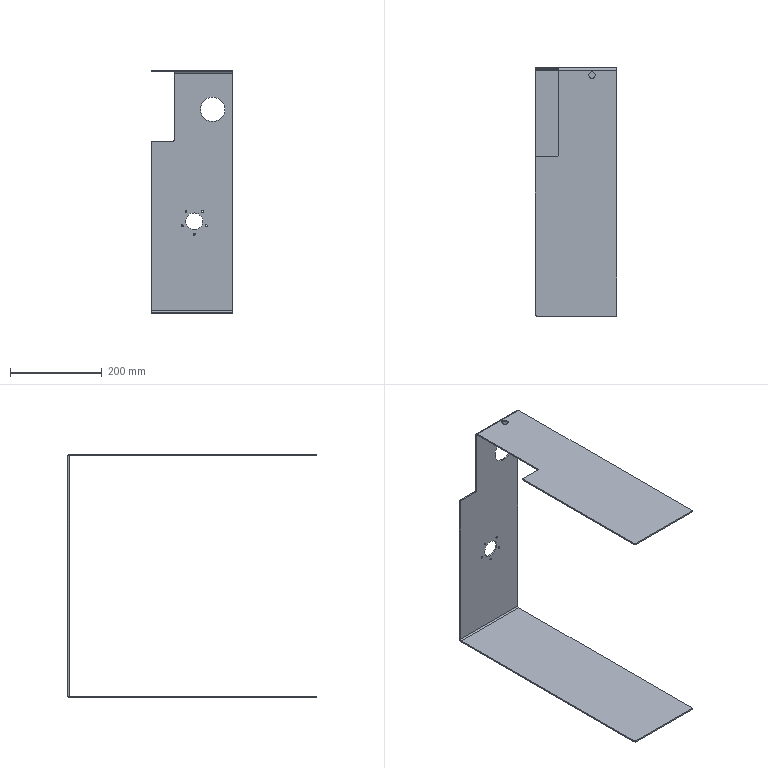Part | SolidWorks | features ICE 3, Fillet 2, FlatPattern 1, HoleWzd 1, SMBaseFlange 1, SheetMetal 1 | 1 solid | 46 faces | box 177 x 542 x 530 mm | volume 789505 mm3 | cylinder 24 | plane 22 | commonest cylinder face diameters 4.2 x10 6 x2 7 x2 8 x2 12 x2 14.2 x2
STEP:
#1=CARTESIAN_POINT('',(93.5,539.,-359.1));
#2=VERTEX_POINT('',#1);
#3=CARTESIAN_POINT('',(93.5,539.,-354.9));
#4=VERTEX_POINT('',#3);
#5=CARTESIAN_POINT('',(93.5,539.,-357.));
#6=DIRECTION('',(0.,1.,0.));
#7=DIRECTION('',(0.,0.,1.));
#8=AXIS2_PLACEMENT_3D('',#5,#6,#7);
#9=CIRCLE('',#8,2.1);
#10=EDGE_CURVE('',#2,#4,#9,.T.);
#11=ORIENTED_EDGE('',*,*,#10,.F.);
#12=CARTESIAN_POINT('',(93.5,542.,-359.1));
#13=VERTEX_POINT('',#12);
#14=CARTESIAN_POINT('',(93.5,542.,-359.1));
#15=DIRECTION('',(0.,1.,0.));
#16=VECTOR('',#15,1000.);
#17=LINE('',#14,#16);
#18=EDGE_CURVE('',#2,#13,#17,.T.);
#19=ORIENTED_EDGE('',*,*,#18,.T.);
#20=CARTESIAN_POINT('',(93.5,542.,-354.9));
#21=VERTEX_POINT('',#20);
#22=CARTESIAN_POINT('',(93.5,542.,-357.));
#23=DIRECTION('',(0.,1.,0.));
#24=DIRECTION('',(0.,0.,1.));
#25=AXIS2_PLACEMENT_3D('',#22,#23,#24);
#26=CIRCLE('',#25,2.1);
#27=EDGE_CURVE('',#13,#21,#26,.T.);
#28=ORIENTED_EDGE('',*,*,#27,.T.);
#29=CARTESIAN_POINT('',(93.5,542.,-354.9));
#30=DIRECTION('',(0.,1.,0.));
#31=VECTOR('',#30,1000.);
#32=LINE('',#29,#31);
#33=EDGE_CURVE('',#4,#21,#32,.T.);
#34=ORIENTED_EDGE('',*,*,#33,.F.);
#35=EDGE_LOOP('',(#11,#19,#28,#34));
#36=FACE_OUTER_BOUND('',#35,.T.);
#37=CARTESIAN_POINT('',(93.5,542.,-357.));
#38=DIRECTION('',(0.,1.,0.));
#39=DIRECTION('',(0.,0.,1.));
#40=AXIS2_PLACEMENT_3D('',#37,#38,#39);
#41=CYLINDRICAL_SURFACE('',#40,2.1);
#42=ADVANCED_FACE('',(#36),#41,.F.);
#43=CARTESIAN_POINT('',(119.811,539.,-340.677));
#44=VERTEX_POINT('',#43);
#45=CARTESIAN_POINT('',(119.811,539.,-336.477));
#46=VERTEX_POINT('',#45);
#47=CARTESIAN_POINT('',(119.811,539.,-338.577));
#48=DIRECTION('',(0.,1.,0.));
#49=DIRECTION('',(0.,0.,1.));
#50=AXIS2_PLACEMENT_3D('',#47,#48,#49);
#51=CIRCLE('',#50,2.1);
#52=EDGE_CURVE('',#44,#46,#51,.T.);
#53=ORIENTED_EDGE('',*,*,#52,.F.);
#54=CARTESIAN_POINT('',(119.811,542.,-340.677));
#55=VERTEX_POINT('',#54);
#56=CARTESIAN_POINT('',(119.811,542.,-340.677));
#57=DIRECTION('',(0.,1.,0.));
#58=VECTOR('',#57,1000.);
#59=LINE('',#56,#58);
#60=EDGE_CURVE('',#44,#55,#59,.T.);
#61=ORIENTED_EDGE('',*,*,#60,.T.);
#62=CARTESIAN_POINT('',(119.811,542.,-336.477));
#63=VERTEX_POINT('',#62);
#64=CARTESIAN_POINT('',(119.811,542.,-338.577));
#65=DIRECTION('',(0.,1.,0.));
#66=DIRECTION('',(0.,0.,1.));
#67=AXIS2_PLACEMENT_3D('',#64,#65,#66);
#68=CIRCLE('',#67,2.1);
#69=EDGE_CURVE('',#55,#63,#68,.T.);
#70=ORIENTED_EDGE('',*,*,#69,.T.);
#71=CARTESIAN_POINT('',(119.811,542.,-336.477));
#72=DIRECTION('',(0.,1.,0.));
#73=VECTOR('',#72,1000.);
#74=LINE('',#71,#73);
#75=EDGE_CURVE('',#46,#63,#74,.T.);
#76=ORIENTED_EDGE('',*,*,#75,.F.);
#77=EDGE_LOOP('',(#53,#61,#70,#76));
#78=FACE_OUTER_BOUND('',#77,.T.);
#79=CARTESIAN_POINT('',(119.811,542.,-338.577));
#80=DIRECTION('',(0.,1.,0.));
#81=DIRECTION('',(0.,0.,1.));
#82=AXIS2_PLACEMENT_3D('',#79,#80,#81);
#83=CYLINDRICAL_SURFACE('',#82,2.1);
#84=ADVANCED_FACE('',(#78),#83,.F.);
#85=CARTESIAN_POINT('',(111.498,539.,-309.651));
#86=VERTEX_POINT('',#85);
#87=CARTESIAN_POINT('',(111.498,539.,-305.451));
#88=VERTEX_POINT('',#87);
#89=CARTESIAN_POINT('',(111.498,539.,-307.551));
#90=DIRECTION('',(0.,1.,0.));
#91=DIRECTION('',(0.,0.,1.));
#92=AXIS2_PLACEMENT_3D('',#89,#90,#91);
#93=CIRCLE('',#92,2.1);
#94=EDGE_CURVE('',#86,#88,#93,.T.);
#95=ORIENTED_EDGE('',*,*,#94,.F.);
#96=CARTESIAN_POINT('',(111.498,542.,-309.651));
#97=VERTEX_POINT('',#96);
#98=CARTESIAN_POINT('',(111.498,542.,-309.651));
#99=DIRECTION('',(0.,1.,0.));
#100=VECTOR('',#99,1000.);
#101=LINE('',#98,#100);
#102=EDGE_CURVE('',#86,#97,#101,.T.);
#103=ORIENTED_EDGE('',*,*,#102,.T.);
#104=CARTESIAN_POINT('',(111.498,542.,-305.451));
#105=VERTEX_POINT('',#104);
#106=CARTESIAN_POINT('',(111.498,542.,-307.551));
#107=DIRECTION('',(0.,1.,0.));
#108=DIRECTION('',(0.,0.,1.));
#109=AXIS2_PLACEMENT_3D('',#106,#107,#108);
#110=CIRCLE('',#109,2.1);
#111=EDGE_CURVE('',#97,#105,#110,.T.);
#112=ORIENTED_EDGE('',*,*,#111,.T.);
#113=CARTESIAN_POINT('',(111.498,542.,-305.451));
#114=DIRECTION('',(0.,1.,0.));
#115=VECTOR('',#114,1000.);
#116=LINE('',#113,#115);
#117=EDGE_CURVE('',#88,#105,#116,.T.);
#118=ORIENTED_EDGE('',*,*,#117,.F.);
#119=EDGE_LOOP('',(#95,#103,#112,#118));
#120=FACE_OUTER_BOUND('',#119,.T.);
#121=CARTESIAN_POINT('',(111.498,542.,-307.551));
#122=DIRECTION('',(0.,1.,0.));
#123=DIRECTION('',(0.,0.,1.));
#124=AXIS2_PLACEMENT_3D('',#121,#122,#123);
#125=CYLINDRICAL_SURFACE('',#124,2.1);
#126=ADVANCED_FACE('',(#120),#125,.F.);
#127=CARTESIAN_POINT('',(75.502,539.,-309.651));
#128=VERTEX_POINT('',#127);
#129=CARTESIAN_POINT('',(75.502,539.,-305.451));
#130=VERTEX_POINT('',#129);
#131=CARTESIAN_POINT('',(75.502,539.,-307.551));
#132=DIRECTION('',(0.,1.,0.));
#133=DIRECTION('',(0.,0.,1.));
#134=AXIS2_PLACEMENT_3D('',#131,#132,#133);
#135=CIRCLE('',#134,2.1);
#136=EDGE_CURVE('',#128,#130,#135,.T.);
#137=ORIENTED_EDGE('',*,*,#136,.F.);
#138=CARTESIAN_POINT('',(75.502,542.,-309.651));
#139=VERTEX_POINT('',#138);
#140=CARTESIAN_POINT('',(75.502,542.,-309.651));
#141=DIRECTION('',(0.,1.,0.));
#142=VECTOR('',#141,1000.);
#143=LINE('',#140,#142);
#144=EDGE_CURVE('',#128,#139,#143,.T.);
#145=ORIENTED_EDGE('',*,*,#144,.T.);
#146=CARTESIAN_POINT('',(75.502,542.,-305.451));
#147=VERTEX_POINT('',#146);
#148=CARTESIAN_POINT('',(75.502,542.,-307.551));
#149=DIRECTION('',(0.,1.,0.));
#150=DIRECTION('',(0.,0.,1.));
#151=AXIS2_PLACEMENT_3D('',#148,#149,#150);
#152=CIRCLE('',#151,2.1);
#153=EDGE_CURVE('',#139,#147,#152,.T.);
#154=ORIENTED_EDGE('',*,*,#153,.T.);
#155=CARTESIAN_POINT('',(75.502,542.,-305.451));
#156=DIRECTION('',(0.,1.,0.));
#157=VECTOR('',#156,1000.);
#158=LINE('',#155,#157);
#159=EDGE_CURVE('',#130,#147,#158,.T.);
#160=ORIENTED_EDGE('',*,*,#159,.F.);
#161=EDGE_LOOP('',(#137,#145,#154,#160));
#162=FACE_OUTER_BOUND('',#161,.T.);
#163=CARTESIAN_POINT('',(75.502,542.,-307.551));
#164=DIRECTION('',(0.,1.,0.));
#165=DIRECTION('',(0.,0.,1.));
#166=AXIS2_PLACEMENT_3D('',#163,#164,#165);
#167=CYLINDRICAL_SURFACE('',#166,2.1);
#168=ADVANCED_FACE('',(#162),#167,.F.);
#169=CARTESIAN_POINT('',(67.189,539.,-340.677));
#170=VERTEX_POINT('',#169);
#171=CARTESIAN_POINT('',(67.189,539.,-336.477));
#172=VERTEX_POINT('',#171);
#173=CARTESIAN_POINT('',(67.189,539.,-338.577));
#174=DIRECTION('',(0.,1.,0.));
#175=DIRECTION('',(0.,0.,1.));
#176=AXIS2_PLACEMENT_3D('',#173,#174,#175);
#177=CIRCLE('',#176,2.1);
#178=EDGE_CURVE('',#170,#172,#177,.T.);
#179=ORIENTED_EDGE('',*,*,#178,.F.);
#180=CARTESIAN_POINT('',(67.189,542.,-340.677));
#181=VERTEX_POINT('',#180);
#182=CARTESIAN_POINT('',(67.189,542.,-340.677));
#183=DIRECTION('',(0.,1.,0.));
#184=VECTOR('',#183,1000.);
#185=LINE('',#182,#184);
#186=EDGE_CURVE('',#170,#181,#185,.T.);
#187=ORIENTED_EDGE('',*,*,#186,.T.);
#188=CARTESIAN_POINT('',(67.189,542.,-336.477));
#189=VERTEX_POINT('',#188);
#190=CARTESIAN_POINT('',(67.189,542.,-338.577));
#191=DIRECTION('',(0.,1.,0.));
#192=DIRECTION('',(0.,0.,1.));
#193=AXIS2_PLACEMENT_3D('',#190,#191,#192);
#194=CIRCLE('',#193,2.1);
#195=EDGE_CURVE('',#181,#189,#194,.T.);
#196=ORIENTED_EDGE('',*,*,#195,.T.);
#197=CARTESIAN_POINT('',(67.189,542.,-336.477));
#198=DIRECTION('',(0.,1.,0.));
#199=VECTOR('',#198,1000.);
#200=LINE('',#197,#199);
#201=EDGE_CURVE('',#172,#189,#200,.T.);
#202=ORIENTED_EDGE('',*,*,#201,.F.);
#203=EDGE_LOOP('',(#179,#187,#196,#202));
#204=FACE_OUTER_BOUND('',#203,.T.);
#205=CARTESIAN_POINT('',(67.189,542.,-338.577));
#206=DIRECTION('',(0.,1.,0.));
#207=DIRECTION('',(0.,0.,1.));
#208=AXIS2_PLACEMENT_3D('',#205,#206,#207);
#209=CYLINDRICAL_SURFACE('',#208,2.1);
#210=ADVANCED_FACE('',(#204),#209,.F.);
#211=CARTESIAN_POINT('',(133.5,539.,-58.5));
#212=VERTEX_POINT('',#211);
#213=CARTESIAN_POINT('',(133.5,539.,-111.5));
#214=VERTEX_POINT('',#213);
#215=CARTESIAN_POINT('',(133.5,539.,-85.));
#216=DIRECTION('',(0.,-1.,0.));
#217=DIRECTION('',(0.,0.,1.));
#218=AXIS2_PLACEMENT_3D('',#215,#216,#217);
#219=CIRCLE('',#218,26.5);
#220=EDGE_CURVE('',#212,#214,#219,.T.);
#221=ORIENTED_EDGE('',*,*,#220,.T.);
#222=CARTESIAN_POINT('',(133.5,542.,-111.5));
#223=VERTEX_POINT('',#222);
#224=CARTESIAN_POINT('',(133.5,-0.001,-111.5));
#225=DIRECTION('',(0.,1.,0.));
#226=VECTOR('',#225,1000.);
#227=LINE('',#224,#226);
#228=EDGE_CURVE('',#214,#223,#227,.T.);
#229=ORIENTED_EDGE('',*,*,#228,.T.);
#230=CARTESIAN_POINT('',(133.5,542.,-58.5));
#231=VERTEX_POINT('',#230);
#232=CARTESIAN_POINT('',(133.5,542.,-85.));
#233=DIRECTION('',(0.,1.,0.));
#234=DIRECTION('',(0.,0.,1.));
#235=AXIS2_PLACEMENT_3D('',#232,#233,#234);
#236=CIRCLE('',#235,26.5);
#237=EDGE_CURVE('',#223,#231,#236,.T.);
#238=ORIENTED_EDGE('',*,*,#237,.T.);
#239=CARTESIAN_POINT('',(133.5,-0.001,-58.5));
#240=DIRECTION('',(0.,1.,0.));
#241=VECTOR('',#240,1000.);
#242=LINE('',#239,#241);
#243=EDGE_CURVE('',#212,#231,#242,.T.);
#244=ORIENTED_EDGE('',*,*,#243,.F.);
#245=EDGE_LOOP('',(#221,#229,#238,#244));
#246=FACE_OUTER_BOUND('',#245,.T.);
#247=CARTESIAN_POINT('',(133.5,-0.001,-85.));
#248=DIRECTION('',(0.,1.,0.));
#249=DIRECTION('',(0.,0.,1.));
#250=AXIS2_PLACEMENT_3D('',#247,#248,#249);
#251=CYLINDRICAL_SURFACE('',#250,26.5);
#252=ADVANCED_FACE('',(#246),#251,.F.);
#253=CARTESIAN_POINT('',(93.5,539.,-310.5));
#254=VERTEX_POINT('',#253);
#255=CARTESIAN_POINT('',(93.5,539.,-347.5));
#256=VERTEX_POINT('',#255);
#257=CARTESIAN_POINT('',(93.5,539.,-329.));
#258=DIRECTION('',(0.,-1.,0.));
#259=DIRECTION('',(0.,0.,1.));
#260=AXIS2_PLACEMENT_3D('',#257,#258,#259);
#261=CIRCLE('',#260,18.5);
#262=EDGE_CURVE('',#254,#256,#261,.T.);
#263=ORIENTED_EDGE('',*,*,#262,.T.);
#264=CARTESIAN_POINT('',(93.5,542.,-347.5));
#265=VERTEX_POINT('',#264);
#266=CARTESIAN_POINT('',(93.5,-0.001,-347.5));
#267=DIRECTION('',(0.,1.,0.));
#268=VECTOR('',#267,1000.);
#269=LINE('',#266,#268);
#270=EDGE_CURVE('',#256,#265,#269,.T.);
#271=ORIENTED_EDGE('',*,*,#270,.T.);
#272=CARTESIAN_POINT('',(93.5,542.,-310.5));
#273=VERTEX_POINT('',#272);
#274=CARTESIAN_POINT('',(93.5,542.,-329.));
#275=DIRECTION('',(0.,1.,0.));
#276=DIRECTION('',(0.,0.,1.));
#277=AXIS2_PLACEMENT_3D('',#274,#275,#276);
#278=CIRCLE('',#277,18.5);
#279=EDGE_CURVE('',#265,#273,#278,.T.);
#280=ORIENTED_EDGE('',*,*,#279,.T.);
#281=CARTESIAN_POINT('',(93.5,-0.001,-310.5));
#282=DIRECTION('',(0.,1.,0.));
#283=VECTOR('',#282,1000.);
#284=LINE('',#281,#283);
#285=EDGE_CURVE('',#254,#273,#284,.T.);
#286=ORIENTED_EDGE('',*,*,#285,.F.);
#287=EDGE_LOOP('',(#263,#271,#280,#286));
#288=FACE_OUTER_BOUND('',#287,.T.);
#289=CARTESIAN_POINT('',(93.5,-0.001,-329.));
#290=DIRECTION('',(0.,1.,0.));
#291=DIRECTION('',(0.,0.,1.));
#292=AXIS2_PLACEMENT_3D('',#289,#290,#291);
#293=CYLINDRICAL_SURFACE('',#292,18.5);
#294=ADVANCED_FACE('',(#288),#293,.F.);
#295=CARTESIAN_POINT('',(130.6,525.,-3.));
#296=VERTEX_POINT('',#295);
#297=CARTESIAN_POINT('',(116.4,525.,-3.));
#298=VERTEX_POINT('',#297);
#299=CARTESIAN_POINT('',(123.5,525.,-3.));
#300=DIRECTION('',(0.,0.,-1.));
#301=DIRECTION('',(1.,0.,0.));
#302=AXIS2_PLACEMENT_3D('',#299,#300,#301);
#303=CIRCLE('',#302,7.1);
#304=EDGE_CURVE('',#296,#298,#303,.T.);
#305=ORIENTED_EDGE('',*,*,#304,.T.);
#306=CARTESIAN_POINT('',(116.4,525.,0.));
#307=VERTEX_POINT('',#306);
#308=CARTESIAN_POINT('',(116.4,525.,-530.001));
#309=DIRECTION('',(0.,0.,1.));
#310=VECTOR('',#309,1000.);
#311=LINE('',#308,#310);
#312=EDGE_CURVE('',#298,#307,#311,.T.);
#313=ORIENTED_EDGE('',*,*,#312,.T.);
#314=CARTESIAN_POINT('',(130.6,525.,0.));
#315=VERTEX_POINT('',#314);
#316=CARTESIAN_POINT('',(123.5,525.,0.));
#317=DIRECTION('',(0.,0.,1.));
#318=DIRECTION('',(1.,0.,0.));
#319=AXIS2_PLACEMENT_3D('',#316,#317,#318);
#320=CIRCLE('',#319,7.1);
#321=EDGE_CURVE('',#307,#315,#320,.T.);
#322=ORIENTED_EDGE('',*,*,#321,.T.);
#323=CARTESIAN_POINT('',(130.6,525.,-530.001));
#324=DIRECTION('',(0.,0.,1.));
#325=VECTOR('',#324,1000.);
#326=LINE('',#323,#325);
#327=EDGE_CURVE('',#296,#315,#326,.T.);
#328=ORIENTED_EDGE('',*,*,#327,.F.);
#329=EDGE_LOOP('',(#305,#313,#322,#328));
#330=FACE_OUTER_BOUND('',#329,.T.);
#331=CARTESIAN_POINT('',(123.5,525.,-530.001));
#332=DIRECTION('',(0.,0.,1.));
#333=DIRECTION('',(1.,0.,0.));
#334=AXIS2_PLACEMENT_3D('',#331,#332,#333);
#335=CYLINDRICAL_SURFACE('',#334,7.1);
#336=ADVANCED_FACE('',(#330),#335,.F.);
#337=CARTESIAN_POINT('',(50.,542.,-6.));
#338=VERTEX_POINT('',#337);
#339=CARTESIAN_POINT('',(50.,542.,-151.5));
#340=VERTEX_POINT('',#339);
#341=CARTESIAN_POINT('',(50.,542.,-155.));
#342=DIRECTION('',(0.,0.,-1.));
#343=VECTOR('',#342,1000.);
#344=LINE('',#341,#343);
#345=EDGE_CURVE('',#338,#340,#344,.T.);
#346=ORIENTED_EDGE('',*,*,#345,.T.);
#347=CARTESIAN_POINT('',(50.,539.,-151.5));
#348=VERTEX_POINT('',#347);
#349=CARTESIAN_POINT('',(50.,539.,-151.5));
#350=DIRECTION('',(0.,-1.,0.));
#351=VECTOR('',#350,1000.);
#352=LINE('',#349,#351);
#353=EDGE_CURVE('',#340,#348,#352,.T.);
#354=ORIENTED_EDGE('',*,*,#353,.T.);
#355=CARTESIAN_POINT('',(50.,539.,-6.));
#356=VERTEX_POINT('',#355);
#357=CARTESIAN_POINT('',(50.,539.,0.));
#358=DIRECTION('',(0.,0.,-1.));
#359=VECTOR('',#358,1000.);
#360=LINE('',#357,#359);
#361=EDGE_CURVE('',#356,#348,#360,.T.);
#362=ORIENTED_EDGE('',*,*,#361,.F.);
#363=CARTESIAN_POINT('',(50.,539.,-6.));
#364=DIRECTION('',(0.,1.,0.));
#365=VECTOR('',#364,1000.);
#366=LINE('',#363,#365);
#367=EDGE_CURVE('',#356,#338,#366,.T.);
#368=ORIENTED_EDGE('',*,*,#367,.T.);
#369=EDGE_LOOP('',(#346,#354,#362,#368));
#370=FACE_OUTER_BOUND('',#369,.T.);
#371=CARTESIAN_POINT('',(50.,347.,-155.));
#372=DIRECTION('',(1.,0.,0.));
#373=DIRECTION('',(0.,0.,-1.));
#374=AXIS2_PLACEMENT_3D('',#371,#372,#373);
#375=PLANE('',#374);
#376=ADVANCED_FACE('',(#370),#375,.F.);
#377=CARTESIAN_POINT('',(50.,350.5,-3.));
#378=VERTEX_POINT('',#377);
#379=CARTESIAN_POINT('',(50.,536.,-3.));
#380=VERTEX_POINT('',#379);
#381=CARTESIAN_POINT('',(50.,0.,-3.));
#382=DIRECTION('',(0.,1.,0.));
#383=VECTOR('',#382,1000.);
#384=LINE('',#381,#383);
#385=EDGE_CURVE('',#378,#380,#384,.T.);
#386=ORIENTED_EDGE('',*,*,#385,.F.);
#387=CARTESIAN_POINT('',(50.,350.5,0.));
#388=VERTEX_POINT('',#387);
#389=CARTESIAN_POINT('',(50.,350.5,0.));
#390=DIRECTION('',(0.,0.,1.));
#391=VECTOR('',#390,1000.);
#392=LINE('',#389,#391);
#393=EDGE_CURVE('',#378,#388,#392,.T.);
#394=ORIENTED_EDGE('',*,*,#393,.T.);
#395=CARTESIAN_POINT('',(50.,536.,0.));
#396=VERTEX_POINT('',#395);
#397=CARTESIAN_POINT('',(50.,347.,0.));
#398=DIRECTION('',(0.,1.,0.));
#399=VECTOR('',#398,1000.);
#400=LINE('',#397,#399);
#401=EDGE_CURVE('',#388,#396,#400,.T.);
#402=ORIENTED_EDGE('',*,*,#401,.T.);
#403=CARTESIAN_POINT('',(50.,536.,0.));
#404=DIRECTION('',(0.,0.,-1.));
#405=VECTOR('',#404,1000.);
#406=LINE('',#403,#405);
#407=EDGE_CURVE('',#396,#380,#406,.T.);
#408=ORIENTED_EDGE('',*,*,#407,.T.);
#409=EDGE_LOOP('',(#386,#394,#402,#408));
#410=FACE_OUTER_BOUND('',#409,.T.);
#411=CARTESIAN_POINT('',(50.,347.,-155.));
#412=DIRECTION('',(1.,0.,0.));
#413=DIRECTION('',(0.,0.,-1.));
#414=AXIS2_PLACEMENT_3D('',#411,#412,#413);
#415=PLANE('',#414);
#416=ADVANCED_FACE('',(#410),#415,.F.);
#417=CARTESIAN_POINT('',(177.,542.,-6.));
#418=VERTEX_POINT('',#417);
#419=CARTESIAN_POINT('',(177.,539.,-6.));
#420=VERTEX_POINT('',#419);
#421=CARTESIAN_POINT('',(177.,542.,-6.));
#422=DIRECTION('',(0.,-1.,0.));
#423=VECTOR('',#422,1000.);
#424=LINE('',#421,#423);
#425=EDGE_CURVE('',#418,#420,#424,.T.);
#426=ORIENTED_EDGE('',*,*,#425,.F.);
#427=CARTESIAN_POINT('',(177.,536.,0.));
#428=VERTEX_POINT('',#427);
#429=CARTESIAN_POINT('',(177.,536.,-6.));
#430=DIRECTION('',(-1.,0.,0.));
#431=DIRECTION('',(0.,0.,-1.));
#432=AXIS2_PLACEMENT_3D('',#429,#430,#431);
#433=CIRCLE('',#432,6.);
#434=EDGE_CURVE('',#428,#418,#433,.T.);
#435=ORIENTED_EDGE('',*,*,#434,.F.);
#436=CARTESIAN_POINT('',(177.,536.,-3.));
#437=VERTEX_POINT('',#436);
#438=CARTESIAN_POINT('',(177.,536.,-3.));
#439=DIRECTION('',(0.,0.,1.));
#440=VECTOR('',#439,1000.);
#441=LINE('',#438,#440);
#442=EDGE_CURVE('',#437,#428,#441,.T.);
#443=ORIENTED_EDGE('',*,*,#442,.F.);
#444=CARTESIAN_POINT('',(177.,536.,-6.));
#445=DIRECTION('',(-1.,0.,0.));
#446=DIRECTION('',(0.,0.,-1.));
#447=AXIS2_PLACEMENT_3D('',#444,#445,#446);
#448=CIRCLE('',#447,3.);
#449=EDGE_CURVE('',#437,#420,#448,.T.);
#450=ORIENTED_EDGE('',*,*,#449,.T.);
#451=EDGE_LOOP('',(#426,#435,#443,#450));
#452=FACE_OUTER_BOUND('',#451,.T.);
#453=CARTESIAN_POINT('',(177.,542.,-6.));
#454=DIRECTION('',(1.,0.,0.));
#455=DIRECTION('',(0.,0.,-1.));
#456=AXIS2_PLACEMENT_3D('',#453,#454,#455);
#457=PLANE('',#456);
#458=ADVANCED_FACE('',(#452),#457,.T.);
#459=CARTESIAN_POINT('',(177.,542.,-524.));
#460=VERTEX_POINT('',#459);
#461=CARTESIAN_POINT('',(177.,542.,0.));
#462=DIRECTION('',(0.,0.,-1.));
#463=VECTOR('',#462,1000.);
#464=LINE('',#461,#463);
#465=EDGE_CURVE('',#418,#460,#464,.T.);
#466=ORIENTED_EDGE('',*,*,#465,.F.);
#467=ORIENTED_EDGE('',*,*,#425,.T.);
#468=CARTESIAN_POINT('',(177.,539.,-524.));
#469=VERTEX_POINT('',#468);
#470=CARTESIAN_POINT('',(177.,539.,0.));
#471=DIRECTION('',(0.,0.,-1.));
#472=VECTOR('',#471,1000.);
#473=LINE('',#470,#472);
#474=EDGE_CURVE('',#420,#469,#473,.T.);
#475=ORIENTED_EDGE('',*,*,#474,.T.);
#476=CARTESIAN_POINT('',(177.,539.,-524.));
#477=DIRECTION('',(0.,1.,0.));
#478=VECTOR('',#477,1000.);
#479=LINE('',#476,#478);
#480=EDGE_CURVE('',#469,#460,#479,.T.);
#481=ORIENTED_EDGE('',*,*,#480,.T.);
#482=EDGE_LOOP('',(#466,#467,#475,#481));
#483=FACE_OUTER_BOUND('',#482,.T.);
#484=CARTESIAN_POINT('',(177.,536.,-3.));
#485=DIRECTION('',(1.,0.,0.));
#486=DIRECTION('',(0.,0.,-1.));
#487=AXIS2_PLACEMENT_3D('',#484,#485,#486);
#488=PLANE('',#487);
#489=ADVANCED_FACE('',(#483),#488,.T.);
#490=CARTESIAN_POINT('',(0.,4.,-3.));
#491=VERTEX_POINT('',#490);
#492=CARTESIAN_POINT('',(0.,347.,-3.));
#493=VERTEX_POINT('',#492);
#494=CARTESIAN_POINT('',(0.,0.,-3.));
#495=DIRECTION('',(0.,1.,0.));
#496=VECTOR('',#495,1000.);
#497=LINE('',#494,#496);
#498=EDGE_CURVE('',#491,#493,#497,.T.);
#499=ORIENTED_EDGE('',*,*,#498,.F.);
#500=CARTESIAN_POINT('',(0.,4.,0.));
#501=VERTEX_POINT('',#500);
#502=CARTESIAN_POINT('',(0.,4.,-6.));
#503=DIRECTION('',(0.,0.,1.));
#504=VECTOR('',#503,1000.);
#505=LINE('',#502,#504);
#506=EDGE_CURVE('',#491,#501,#505,.T.);
#507=ORIENTED_EDGE('',*,*,#506,.T.);
#508=CARTESIAN_POINT('',(0.,347.,0.));
#509=VERTEX_POINT('',#508);
#510=CARTESIAN_POINT('',(0.,0.,0.));
#511=DIRECTION('',(0.,1.,0.));
#512=VECTOR('',#511,1000.);
#513=LINE('',#510,#512);
#514=EDGE_CURVE('',#501,#509,#513,.T.);
#515=ORIENTED_EDGE('',*,*,#514,.T.);
#516=CARTESIAN_POINT('',(0.,347.,0.));
#517=DIRECTION('',(0.,0.,1.));
#518=VECTOR('',#517,1000.);
#519=LINE('',#516,#518);
#520=EDGE_CURVE('',#493,#509,#519,.T.);
#521=ORIENTED_EDGE('',*,*,#520,.F.);
#522=EDGE_LOOP('',(#499,#507,#515,#521));
#523=FACE_OUTER_BOUND('',#522,.T.);
#524=CARTESIAN_POINT('',(0.,539.,-6.));
#525=DIRECTION('',(-1.,0.,0.));
#526=DIRECTION('',(0.,0.,1.));
#527=AXIS2_PLACEMENT_3D('',#524,#525,#526);
#528=PLANE('',#527);
#529=ADVANCED_FACE('',(#523),#528,.T.);
#530=CARTESIAN_POINT('',(177.,536.,-530.));
#531=VERTEX_POINT('',#530);
#532=CARTESIAN_POINT('',(177.,536.,-527.));
#533=VERTEX_POINT('',#532);
#534=CARTESIAN_POINT('',(177.,536.,-530.));
#535=DIRECTION('',(0.,0.,1.));
#536=VECTOR('',#535,1000.);
#537=LINE('',#534,#536);
#538=EDGE_CURVE('',#531,#533,#537,.T.);
#539=ORIENTED_EDGE('',*,*,#538,.F.);
#540=CARTESIAN_POINT('',(177.,536.,-524.));
#541=DIRECTION('',(-1.,0.,0.));
#542=DIRECTION('',(0.,0.,-1.));
#543=AXIS2_PLACEMENT_3D('',#540,#541,#542);
#544=CIRCLE('',#543,6.);
#545=EDGE_CURVE('',#460,#531,#544,.T.);
#546=ORIENTED_EDGE('',*,*,#545,.F.);
#547=ORIENTED_EDGE('',*,*,#480,.F.);
#548=CARTESIAN_POINT('',(177.,536.,-524.));
#549=DIRECTION('',(-1.,0.,0.));
#550=DIRECTION('',(0.,0.,-1.));
#551=AXIS2_PLACEMENT_3D('',#548,#549,#550);
#552=CIRCLE('',#551,3.);
#553=EDGE_CURVE('',#469,#533,#552,.T.);
#554=ORIENTED_EDGE('',*,*,#553,.T.);
#555=EDGE_LOOP('',(#539,#546,#547,#554));
#556=FACE_OUTER_BOUND('',#555,.T.);
#557=CARTESIAN_POINT('',(177.,536.,-530.));
#558=DIRECTION('',(1.,0.,0.));
#559=DIRECTION('',(0.,0.,-1.));
#560=AXIS2_PLACEMENT_3D('',#557,#558,#559);
#561=PLANE('',#560);
#562=ADVANCED_FACE('',(#556),#561,.T.);
#563=CARTESIAN_POINT('',(177.,0.,-530.));
#564=VERTEX_POINT('',#563);
#565=CARTESIAN_POINT('',(177.,542.,-530.));
#566=DIRECTION('',(0.,-1.,0.));
#567=VECTOR('',#566,1000.);
#568=LINE('',#565,#567);
#569=EDGE_CURVE('',#531,#564,#568,.T.);
#570=ORIENTED_EDGE('',*,*,#569,.F.);
#571=ORIENTED_EDGE('',*,*,#538,.T.);
#572=CARTESIAN_POINT('',(177.,0.,-527.));
#573=VERTEX_POINT('',#572);
#574=CARTESIAN_POINT('',(177.,542.,-527.));
#575=DIRECTION('',(0.,-1.,0.));
#576=VECTOR('',#575,1000.);
#577=LINE('',#574,#576);
#578=EDGE_CURVE('',#533,#573,#577,.T.);
#579=ORIENTED_EDGE('',*,*,#578,.T.);
#580=CARTESIAN_POINT('',(177.,0.,-530.));
#581=DIRECTION('',(0.,0.,1.));
#582=VECTOR('',#581,1000.);
#583=LINE('',#580,#582);
#584=EDGE_CURVE('',#564,#573,#583,.T.);
#585=ORIENTED_EDGE('',*,*,#584,.F.);
#586=EDGE_LOOP('',(#570,#571,#579,#585));
#587=FACE_OUTER_BOUND('',#586,.T.);
#588=CARTESIAN_POINT('',(177.,539.,-524.));
#589=DIRECTION('',(1.,0.,0.));
#590=DIRECTION('',(0.,0.,-1.));
#591=AXIS2_PLACEMENT_3D('',#588,#589,#590);
#592=PLANE('',#591);
#593=ADVANCED_FACE('',(#587),#592,.T.);
#594=CARTESIAN_POINT('',(0.,542.,-524.));
#595=VERTEX_POINT('',#594);
#596=CARTESIAN_POINT('',(0.,539.,-524.));
#597=VERTEX_POINT('',#596);
#598=CARTESIAN_POINT('',(0.,542.,-524.));
#599=DIRECTION('',(0.,-1.,0.));
#600=VECTOR('',#599,1000.);
#601=LINE('',#598,#600);
#602=EDGE_CURVE('',#595,#597,#601,.T.);
#603=ORIENTED_EDGE('',*,*,#602,.F.);
#604=CARTESIAN_POINT('',(0.,536.,-530.));
#605=VERTEX_POINT('',#604);
#606=CARTESIAN_POINT('',(0.,536.,-524.));
#607=DIRECTION('',(-1.,0.,0.));
#608=DIRECTION('',(0.,0.,-1.));
#609=AXIS2_PLACEMENT_3D('',#606,#607,#608);
#610=CIRCLE('',#609,6.);
#611=EDGE_CURVE('',#595,#605,#610,.T.);
#612=ORIENTED_EDGE('',*,*,#611,.T.);
#613=CARTESIAN_POINT('',(0.,536.,-527.));
#614=VERTEX_POINT('',#613);
#615=CARTESIAN_POINT('',(0.,536.,-527.));
#616=DIRECTION('',(0.,0.,-1.));
#617=VECTOR('',#616,1000.);
#618=LINE('',#615,#617);
#619=EDGE_CURVE('',#614,#605,#618,.T.);
#620=ORIENTED_EDGE('',*,*,#619,.F.);
#621=CARTESIAN_POINT('',(0.,536.,-524.));
#622=DIRECTION('',(-1.,0.,0.));
#623=DIRECTION('',(0.,0.,-1.));
#624=AXIS2_PLACEMENT_3D('',#621,#622,#623);
#625=CIRCLE('',#624,3.);
#626=EDGE_CURVE('',#597,#614,#625,.T.);
#627=ORIENTED_EDGE('',*,*,#626,.F.);
#628=EDGE_LOOP('',(#603,#612,#620,#627));
#629=FACE_OUTER_BOUND('',#628,.T.);
#630=CARTESIAN_POINT('',(0.,542.,-524.));
#631=DIRECTION('',(-1.,0.,0.));
#632=DIRECTION('',(0.,0.,1.));
#633=AXIS2_PLACEMENT_3D('',#630,#631,#632);
#634=PLANE('',#633);
#635=ADVANCED_FACE('',(#629),#634,.T.);
#636=CARTESIAN_POINT('',(0.,539.,-155.));
#637=VERTEX_POINT('',#636);
#638=CARTESIAN_POINT('',(0.,542.,-155.));
#639=VERTEX_POINT('',#638);
#640=CARTESIAN_POINT('',(0.,347.,-155.));
#641=DIRECTION('',(0.,1.,0.));
#642=VECTOR('',#641,1000.);
#643=LINE('',#640,#642);
#644=EDGE_CURVE('',#637,#639,#643,.T.);
#645=ORIENTED_EDGE('',*,*,#644,.T.);
#646=CARTESIAN_POINT('',(0.,542.,0.));
#647=DIRECTION('',(0.,0.,-1.));
#648=VECTOR('',#647,1000.);
#649=LINE('',#646,#648);
#650=EDGE_CURVE('',#639,#595,#649,.T.);
#651=ORIENTED_EDGE('',*,*,#650,.T.);
#652=ORIENTED_EDGE('',*,*,#602,.T.);
#653=CARTESIAN_POINT('',(0.,539.,0.));
#654=DIRECTION('',(0.,0.,-1.));
#655=VECTOR('',#654,1000.);
#656=LINE('',#653,#655);
#657=EDGE_CURVE('',#637,#597,#656,.T.);
#658=ORIENTED_EDGE('',*,*,#657,.F.);
#659=EDGE_LOOP('',(#645,#651,#652,#658));
#660=FACE_OUTER_BOUND('',#659,.T.);
#661=CARTESIAN_POINT('',(0.,536.,-527.));
#662=DIRECTION('',(-1.,0.,0.));
#663=DIRECTION('',(0.,0.,1.));
#664=AXIS2_PLACEMENT_3D('',#661,#662,#663);
#665=PLANE('',#664);
#666=ADVANCED_FACE('',(#660),#665,.T.);
#667=CARTESIAN_POINT('',(0.,4.,-527.));
#668=VERTEX_POINT('',#667);
#669=CARTESIAN_POINT('',(0.,542.,-527.));
#670=DIRECTION('',(0.,-1.,0.));
#671=VECTOR('',#670,1000.);
#672=LINE('',#669,#671);
#673=EDGE_CURVE('',#614,#668,#672,.T.);
#674=ORIENTED_EDGE('',*,*,#673,.T.);
#675=CARTESIAN_POINT('',(4.,0.,-527.));
#676=VERTEX_POINT('',#675);
#677=CARTESIAN_POINT('',(4.,4.,-527.));
#678=DIRECTION('',(0.,0.,1.));
#679=DIRECTION('',(0.,1.,0.));
#680=AXIS2_PLACEMENT_3D('',#677,#678,#679);
#681=CIRCLE('',#680,4.);
#682=EDGE_CURVE('',#668,#676,#681,.T.);
#683=ORIENTED_EDGE('',*,*,#682,.T.);
#684=CARTESIAN_POINT('',(177.,0.,-527.));
#685=DIRECTION('',(-1.,0.,0.));
#686=VECTOR('',#685,1000.);
#687=LINE('',#684,#686);
#688=EDGE_CURVE('',#573,#676,#687,.T.);
#689=ORIENTED_EDGE('',*,*,#688,.F.);
#690=ORIENTED_EDGE('',*,*,#578,.F.);
#691=CARTESIAN_POINT('',(177.,536.,-527.));
#692=DIRECTION('',(-1.,0.,0.));
#693=VECTOR('',#692,1000.);
#694=LINE('',#691,#693);
#695=EDGE_CURVE('',#533,#614,#694,.T.);
#696=ORIENTED_EDGE('',*,*,#695,.T.);
#697=EDGE_LOOP('',(#674,#683,#689,#690,#696));
#698=FACE_OUTER_BOUND('',#697,.T.);
#699=CARTESIAN_POINT('',(177.,542.,-527.));
#700=DIRECTION('',(0.,0.,-1.));
#701=DIRECTION('',(0.,1.,0.));
#702=AXIS2_PLACEMENT_3D('',#699,#700,#701);
#703=PLANE('',#702);
#704=ADVANCED_FACE('',(#698),#703,.F.);
#705=ORIENTED_EDGE('',*,*,#688,.T.);
#706=CARTESIAN_POINT('',(4.,0.,-530.));
#707=VERTEX_POINT('',#706);
#708=CARTESIAN_POINT('',(4.,0.,-530.));
#709=DIRECTION('',(0.,0.,-1.));
#710=VECTOR('',#709,1000.);
#711=LINE('',#708,#710);
#712=EDGE_CURVE('',#676,#707,#711,.T.);
#713=ORIENTED_EDGE('',*,*,#712,.T.);
#714=CARTESIAN_POINT('',(177.,0.,-530.));
#715=DIRECTION('',(-1.,0.,0.));
#716=VECTOR('',#715,1000.);
#717=LINE('',#714,#716);
#718=EDGE_CURVE('',#564,#707,#717,.T.);
#719=ORIENTED_EDGE('',*,*,#718,.F.);
#720=ORIENTED_EDGE('',*,*,#584,.T.);
#721=EDGE_LOOP('',(#705,#713,#719,#720));
#722=FACE_OUTER_BOUND('',#721,.T.);
#723=CARTESIAN_POINT('',(177.,0.,-530.));
#724=DIRECTION('',(0.,-1.,0.));
#725=DIRECTION('',(0.,0.,-1.));
#726=AXIS2_PLACEMENT_3D('',#723,#724,#725);
#727=PLANE('',#726);
#728=ADVANCED_FACE('',(#722),#727,.T.);
#729=ORIENTED_EDGE('',*,*,#718,.T.);
#730=CARTESIAN_POINT('',(0.,4.,-530.));
#731=VERTEX_POINT('',#730);
#732=CARTESIAN_POINT('',(4.,4.,-530.));
#733=DIRECTION('',(0.,0.,-1.));
#734=DIRECTION('',(0.,1.,0.));
#735=AXIS2_PLACEMENT_3D('',#732,#733,#734);
#736=CIRCLE('',#735,4.);
#737=EDGE_CURVE('',#707,#731,#736,.T.);
#738=ORIENTED_EDGE('',*,*,#737,.T.);
#739=CARTESIAN_POINT('',(0.,542.,-530.));
#740=DIRECTION('',(0.,-1.,0.));
#741=VECTOR('',#740,1000.);
#742=LINE('',#739,#741);
#743=EDGE_CURVE('',#605,#731,#742,.T.);
#744=ORIENTED_EDGE('',*,*,#743,.F.);
#745=CARTESIAN_POINT('',(177.,536.,-530.));
#746=DIRECTION('',(-1.,0.,0.));
#747=VECTOR('',#746,1000.);
#748=LINE('',#745,#747);
#749=EDGE_CURVE('',#531,#605,#748,.T.);
#750=ORIENTED_EDGE('',*,*,#749,.F.);
#751=ORIENTED_EDGE('',*,*,#569,.T.);
#752=EDGE_LOOP('',(#729,#738,#744,#750,#751));
#753=FACE_OUTER_BOUND('',#752,.T.);
#754=CARTESIAN_POINT('',(177.,542.,-530.));
#755=DIRECTION('',(0.,0.,-1.));
#756=DIRECTION('',(0.,1.,0.));
#757=AXIS2_PLACEMENT_3D('',#754,#755,#756);
#758=PLANE('',#757);
#759=ADVANCED_FACE('',(#753),#758,.T.);
#760=ORIENTED_EDGE('',*,*,#611,.F.);
#761=CARTESIAN_POINT('',(177.,542.,-524.));
#762=DIRECTION('',(-1.,0.,0.));
#763=VECTOR('',#762,1000.);
#764=LINE('',#761,#763);
#765=EDGE_CURVE('',#460,#595,#764,.T.);
#766=ORIENTED_EDGE('',*,*,#765,.F.);
#767=ORIENTED_EDGE('',*,*,#545,.T.);
#768=ORIENTED_EDGE('',*,*,#749,.T.);
#769=EDGE_LOOP('',(#760,#766,#767,#768));
#770=FACE_OUTER_BOUND('',#769,.T.);
#771=CARTESIAN_POINT('',(177.,536.,-524.));
#772=DIRECTION('',(-1.,0.,0.));
#773=DIRECTION('',(0.,0.,1.));
#774=AXIS2_PLACEMENT_3D('',#771,#772,#773);
#775=CYLINDRICAL_SURFACE('',#774,6.);
#776=ADVANCED_FACE('',(#770),#775,.T.);
#777=CARTESIAN_POINT('',(93.5,542.,-357.));
#778=DIRECTION('',(0.,1.,0.));
#779=DIRECTION('',(0.,0.,1.));
#780=AXIS2_PLACEMENT_3D('',#777,#778,#779);
#781=CIRCLE('',#780,2.1);
#782=EDGE_CURVE('',#21,#13,#781,.T.);
#783=ORIENTED_EDGE('',*,*,#782,.F.);
#784=ORIENTED_EDGE('',*,*,#27,.F.);
#785=EDGE_LOOP('',(#783,#784));
#786=FACE_BOUND('',#785,.T.);
#787=CARTESIAN_POINT('',(119.811,542.,-338.577));
#788=DIRECTION('',(0.,1.,0.));
#789=DIRECTION('',(0.,0.,1.));
#790=AXIS2_PLACEMENT_3D('',#787,#788,#789);
#791=CIRCLE('',#790,2.1);
#792=EDGE_CURVE('',#63,#55,#791,.T.);
#793=ORIENTED_EDGE('',*,*,#792,.F.);
#794=ORIENTED_EDGE('',*,*,#69,.F.);
#795=EDGE_LOOP('',(#793,#794));
#796=FACE_BOUND('',#795,.T.);
#797=CARTESIAN_POINT('',(111.498,542.,-307.551));
#798=DIRECTION('',(0.,1.,0.));
#799=DIRECTION('',(0.,0.,1.));
#800=AXIS2_PLACEMENT_3D('',#797,#798,#799);
#801=CIRCLE('',#800,2.1);
#802=EDGE_CURVE('',#105,#97,#801,.T.);
#803=ORIENTED_EDGE('',*,*,#802,.F.);
#804=ORIENTED_EDGE('',*,*,#111,.F.);
#805=EDGE_LOOP('',(#803,#804));
#806=FACE_BOUND('',#805,.T.);
#807=CARTESIAN_POINT('',(75.502,542.,-307.551));
#808=DIRECTION('',(0.,1.,0.));
#809=DIRECTION('',(0.,0.,1.));
#810=AXIS2_PLACEMENT_3D('',#807,#808,#809);
#811=CIRCLE('',#810,2.1);
#812=EDGE_CURVE('',#147,#139,#811,.T.);
#813=ORIENTED_EDGE('',*,*,#812,.F.);
#814=ORIENTED_EDGE('',*,*,#153,.F.);
#815=EDGE_LOOP('',(#813,#814));
#816=FACE_BOUND('',#815,.T.);
#817=CARTESIAN_POINT('',(67.189,542.,-338.577));
#818=DIRECTION('',(0.,1.,0.));
#819=DIRECTION('',(0.,0.,1.));
#820=AXIS2_PLACEMENT_3D('',#817,#818,#819);
#821=CIRCLE('',#820,2.1);
#822=EDGE_CURVE('',#189,#181,#821,.T.);
#823=ORIENTED_EDGE('',*,*,#822,.F.);
#824=ORIENTED_EDGE('',*,*,#195,.F.);
#825=EDGE_LOOP('',(#823,#824));
#826=FACE_BOUND('',#825,.T.);
#827=CARTESIAN_POINT('',(133.5,542.,-85.));
#828=DIRECTION('',(0.,1.,0.));
#829=DIRECTION('',(0.,0.,1.));
#830=AXIS2_PLACEMENT_3D('',#827,#828,#829);
#831=CIRCLE('',#830,26.5);
#832=EDGE_CURVE('',#231,#223,#831,.T.);
#833=ORIENTED_EDGE('',*,*,#832,.F.);
#834=ORIENTED_EDGE('',*,*,#237,.F.);
#835=EDGE_LOOP('',(#833,#834));
#836=FACE_BOUND('',#835,.T.);
#837=CARTESIAN_POINT('',(93.5,542.,-329.));
#838=DIRECTION('',(0.,1.,0.));
#839=DIRECTION('',(0.,0.,1.));
#840=AXIS2_PLACEMENT_3D('',#837,#838,#839);
#841=CIRCLE('',#840,18.5);
#842=EDGE_CURVE('',#273,#265,#841,.T.);
#843=ORIENTED_EDGE('',*,*,#842,.F.);
#844=ORIENTED_EDGE('',*,*,#279,.F.);
#845=EDGE_LOOP('',(#843,#844));
#846=FACE_BOUND('',#845,.T.);
#847=CARTESIAN_POINT('',(46.5,542.,-155.));
#848=VERTEX_POINT('',#847);
#849=CARTESIAN_POINT('',(0.,542.,-155.));
#850=DIRECTION('',(-1.,0.,0.));
#851=VECTOR('',#850,1000.);
#852=LINE('',#849,#851);
#853=EDGE_CURVE('',#848,#639,#852,.T.);
#854=ORIENTED_EDGE('',*,*,#853,.F.);
#855=CARTESIAN_POINT('',(46.5,542.,-151.5));
#856=DIRECTION('',(0.,-1.,0.));
#857=DIRECTION('',(0.,0.,1.));
#858=AXIS2_PLACEMENT_3D('',#855,#856,#857);
#859=CIRCLE('',#858,3.5);
#860=EDGE_CURVE('',#848,#340,#859,.T.);
#861=ORIENTED_EDGE('',*,*,#860,.T.);
#862=ORIENTED_EDGE('',*,*,#345,.F.);
#863=CARTESIAN_POINT('',(177.,542.,-6.));
#864=DIRECTION('',(-1.,0.,0.));
#865=VECTOR('',#864,1000.);
#866=LINE('',#863,#865);
#867=EDGE_CURVE('',#418,#338,#866,.T.);
#868=ORIENTED_EDGE('',*,*,#867,.F.);
#869=ORIENTED_EDGE('',*,*,#465,.T.);
#870=ORIENTED_EDGE('',*,*,#765,.T.);
#871=ORIENTED_EDGE('',*,*,#650,.F.);
#872=EDGE_LOOP('',(#854,#861,#862,#868,#869,#870,#871));
#873=FACE_OUTER_BOUND('',#872,.T.);
#874=CARTESIAN_POINT('',(177.,542.,0.));
#875=DIRECTION('',(0.,1.,0.));
#876=DIRECTION('',(0.,0.,1.));
#877=AXIS2_PLACEMENT_3D('',#874,#875,#876);
#878=PLANE('',#877);
#879=ADVANCED_FACE('',(#786,#796,#806,#816,#826,#836,#846,#873),#878,.T.);
#880=CARTESIAN_POINT('',(50.,536.,-6.));
#881=DIRECTION('',(-1.,0.,0.));
#882=DIRECTION('',(0.,0.,-1.));
#883=AXIS2_PLACEMENT_3D('',#880,#881,#882);
#884=CIRCLE('',#883,6.);
#885=EDGE_CURVE('',#396,#338,#884,.T.);
#886=ORIENTED_EDGE('',*,*,#885,.F.);
#887=CARTESIAN_POINT('',(177.,536.,0.));
#888=DIRECTION('',(-1.,0.,0.));
#889=VECTOR('',#888,1000.);
#890=LINE('',#887,#889);
#891=EDGE_CURVE('',#428,#396,#890,.T.);
#892=ORIENTED_EDGE('',*,*,#891,.F.);
#893=ORIENTED_EDGE('',*,*,#434,.T.);
#894=ORIENTED_EDGE('',*,*,#867,.T.);
#895=EDGE_LOOP('',(#886,#892,#893,#894));
#896=FACE_OUTER_BOUND('',#895,.T.);
#897=CARTESIAN_POINT('',(177.,536.,-6.));
#898=DIRECTION('',(-1.,0.,0.));
#899=DIRECTION('',(0.,0.,1.));
#900=AXIS2_PLACEMENT_3D('',#897,#898,#899);
#901=CYLINDRICAL_SURFACE('',#900,6.);
#902=ADVANCED_FACE('',(#896),#901,.T.);
#903=CARTESIAN_POINT('',(123.5,525.,0.));
#904=DIRECTION('',(0.,0.,1.));
#905=DIRECTION('',(1.,0.,0.));
#906=AXIS2_PLACEMENT_3D('',#903,#904,#905);
#907=CIRCLE('',#906,7.1);
#908=EDGE_CURVE('',#315,#307,#907,.T.);
#909=ORIENTED_EDGE('',*,*,#908,.F.);
#910=ORIENTED_EDGE('',*,*,#321,.F.);
#911=EDGE_LOOP('',(#909,#910));
#912=FACE_BOUND('',#911,.T.);
#913=ORIENTED_EDGE('',*,*,#514,.F.);
#914=CARTESIAN_POINT('',(4.,0.,0.));
#915=VERTEX_POINT('',#914);
#916=CARTESIAN_POINT('',(4.,4.,0.));
#917=DIRECTION('',(0.,0.,1.));
#918=DIRECTION('',(1.,0.,0.));
#919=AXIS2_PLACEMENT_3D('',#916,#917,#918);
#920=CIRCLE('',#919,4.);
#921=EDGE_CURVE('',#501,#915,#920,.T.);
#922=ORIENTED_EDGE('',*,*,#921,.T.);
#923=CARTESIAN_POINT('',(177.,0.,0.));
#924=VERTEX_POINT('',#923);
#925=CARTESIAN_POINT('',(177.,0.,0.));
#926=DIRECTION('',(-1.,0.,0.));
#927=VECTOR('',#926,1000.);
#928=LINE('',#925,#927);
#929=EDGE_CURVE('',#924,#915,#928,.T.);
#930=ORIENTED_EDGE('',*,*,#929,.F.);
#931=CARTESIAN_POINT('',(177.,0.,0.));
#932=DIRECTION('',(0.,1.,0.));
#933=VECTOR('',#932,1000.);
#934=LINE('',#931,#933);
#935=EDGE_CURVE('',#924,#428,#934,.T.);
#936=ORIENTED_EDGE('',*,*,#935,.T.);
#937=ORIENTED_EDGE('',*,*,#891,.T.);
#938=ORIENTED_EDGE('',*,*,#401,.F.);
#939=CARTESIAN_POINT('',(46.5,347.,0.));
#940=VERTEX_POINT('',#939);
#941=CARTESIAN_POINT('',(46.5,350.5,0.));
#942=DIRECTION('',(0.,0.,-1.));
#943=DIRECTION('',(1.,0.,0.));
#944=AXIS2_PLACEMENT_3D('',#941,#942,#943);
#945=CIRCLE('',#944,3.5);
#946=EDGE_CURVE('',#388,#940,#945,.T.);
#947=ORIENTED_EDGE('',*,*,#946,.T.);
#948=CARTESIAN_POINT('',(50.,347.,0.));
#949=DIRECTION('',(1.,0.,0.));
#950=VECTOR('',#949,1000.);
#951=LINE('',#948,#950);
#952=EDGE_CURVE('',#509,#940,#951,.T.);
#953=ORIENTED_EDGE('',*,*,#952,.F.);
#954=EDGE_LOOP('',(#913,#922,#930,#936,#937,#938,#947,#953));
#955=FACE_OUTER_BOUND('',#954,.T.);
#956=CARTESIAN_POINT('',(177.,0.,0.));
#957=DIRECTION('',(0.,0.,1.));
#958=DIRECTION('',(1.,0.,0.));
#959=AXIS2_PLACEMENT_3D('',#956,#957,#958);
#960=PLANE('',#959);
#961=ADVANCED_FACE('',(#912,#955),#960,.T.);
#962=ORIENTED_EDGE('',*,*,#929,.T.);
#963=CARTESIAN_POINT('',(4.,0.,-3.));
#964=VERTEX_POINT('',#963);
#965=CARTESIAN_POINT('',(4.,0.,-3.));
#966=DIRECTION('',(0.,0.,-1.));
#967=VECTOR('',#966,1000.);
#968=LINE('',#965,#967);
#969=EDGE_CURVE('',#915,#964,#968,.T.);
#970=ORIENTED_EDGE('',*,*,#969,.T.);
#971=CARTESIAN_POINT('',(177.,0.,-3.));
#972=VERTEX_POINT('',#971);
#973=CARTESIAN_POINT('',(177.,0.,-3.));
#974=DIRECTION('',(-1.,0.,0.));
#975=VECTOR('',#974,1000.);
#976=LINE('',#973,#975);
#977=EDGE_CURVE('',#972,#964,#976,.T.);
#978=ORIENTED_EDGE('',*,*,#977,.F.);
#979=CARTESIAN_POINT('',(177.,0.,-3.));
#980=DIRECTION('',(0.,0.,1.));
#981=VECTOR('',#980,1000.);
#982=LINE('',#979,#981);
#983=EDGE_CURVE('',#972,#924,#982,.T.);
#984=ORIENTED_EDGE('',*,*,#983,.T.);
#985=EDGE_LOOP('',(#962,#970,#978,#984));
#986=FACE_OUTER_BOUND('',#985,.T.);
#987=CARTESIAN_POINT('',(177.,0.,-3.));
#988=DIRECTION('',(0.,-1.,0.));
#989=DIRECTION('',(0.,0.,-1.));
#990=AXIS2_PLACEMENT_3D('',#987,#988,#989);
#991=PLANE('',#990);
#992=ADVANCED_FACE('',(#986),#991,.T.);
#993=ORIENTED_EDGE('',*,*,#304,.F.);
#994=CARTESIAN_POINT('',(123.5,525.,-3.));
#995=DIRECTION('',(0.,0.,-1.));
#996=DIRECTION('',(1.,0.,0.));
#997=AXIS2_PLACEMENT_3D('',#994,#995,#996);
#998=CIRCLE('',#997,7.1);
#999=EDGE_CURVE('',#298,#296,#998,.T.);
#1000=ORIENTED_EDGE('',*,*,#999,.F.);
#1001=EDGE_LOOP('',(#993,#1000));
#1002=FACE_BOUND('',#1001,.T.);
#1003=ORIENTED_EDGE('',*,*,#977,.T.);
#1004=CARTESIAN_POINT('',(4.,4.,-3.));
#1005=DIRECTION('',(0.,0.,-1.));
#1006=DIRECTION('',(1.,0.,0.));
#1007=AXIS2_PLACEMENT_3D('',#1004,#1005,#1006);
#1008=CIRCLE('',#1007,4.);
#1009=EDGE_CURVE('',#964,#491,#1008,.T.);
#1010=ORIENTED_EDGE('',*,*,#1009,.T.);
#1011=ORIENTED_EDGE('',*,*,#498,.T.);
#1012=CARTESIAN_POINT('',(46.5,347.,-3.));
#1013=VERTEX_POINT('',#1012);
#1014=CARTESIAN_POINT('',(177.,347.,-3.));
#1015=DIRECTION('',(1.,0.,0.));
#1016=VECTOR('',#1015,1000.);
#1017=LINE('',#1014,#1016);
#1018=EDGE_CURVE('',#493,#1013,#1017,.T.);
#1019=ORIENTED_EDGE('',*,*,#1018,.T.);
#1020=CARTESIAN_POINT('',(46.5,350.5,-3.));
#1021=DIRECTION('',(0.,0.,1.));
#1022=DIRECTION('',(1.,0.,0.));
#1023=AXIS2_PLACEMENT_3D('',#1020,#1021,#1022);
#1024=CIRCLE('',#1023,3.5);
#1025=EDGE_CURVE('',#1013,#378,#1024,.T.);
#1026=ORIENTED_EDGE('',*,*,#1025,.T.);
#1027=ORIENTED_EDGE('',*,*,#385,.T.);
#1028=CARTESIAN_POINT('',(177.,536.,-3.));
#1029=DIRECTION('',(-1.,0.,0.));
#1030=VECTOR('',#1029,1000.);
#1031=LINE('',#1028,#1030);
#1032=EDGE_CURVE('',#437,#380,#1031,.T.);
#1033=ORIENTED_EDGE('',*,*,#1032,.F.);
#1034=CARTESIAN_POINT('',(177.,0.,-3.));
#1035=DIRECTION('',(0.,1.,0.));
#1036=VECTOR('',#1035,1000.);
#1037=LINE('',#1034,#1036);
#1038=EDGE_CURVE('',#972,#437,#1037,.T.);
#1039=ORIENTED_EDGE('',*,*,#1038,.F.);
#1040=EDGE_LOOP('',(#1003,#1010,#1011,#1019,#1026,#1027,#1033,#1039));
#1041=FACE_OUTER_BOUND('',#1040,.T.);
#1042=CARTESIAN_POINT('',(177.,0.,-3.));
#1043=DIRECTION('',(0.,0.,1.));
#1044=DIRECTION('',(1.,0.,0.));
#1045=AXIS2_PLACEMENT_3D('',#1042,#1043,#1044);
#1046=PLANE('',#1045);
#1047=ADVANCED_FACE('',(#1002,#1041),#1046,.F.);
#1048=ORIENTED_EDGE('',*,*,#1032,.T.);
#1049=CARTESIAN_POINT('',(50.,536.,-6.));
#1050=DIRECTION('',(-1.,0.,0.));
#1051=DIRECTION('',(0.,0.,-1.));
#1052=AXIS2_PLACEMENT_3D('',#1049,#1050,#1051);
#1053=CIRCLE('',#1052,3.);
#1054=EDGE_CURVE('',#380,#356,#1053,.T.);
#1055=ORIENTED_EDGE('',*,*,#1054,.T.);
#1056=CARTESIAN_POINT('',(177.,539.,-6.));
#1057=DIRECTION('',(-1.,0.,0.));
#1058=VECTOR('',#1057,1000.);
#1059=LINE('',#1056,#1058);
#1060=EDGE_CURVE('',#420,#356,#1059,.T.);
#1061=ORIENTED_EDGE('',*,*,#1060,.F.);
#1062=ORIENTED_EDGE('',*,*,#449,.F.);
#1063=EDGE_LOOP('',(#1048,#1055,#1061,#1062));
#1064=FACE_OUTER_BOUND('',#1063,.T.);
#1065=CARTESIAN_POINT('',(177.,536.,-6.));
#1066=DIRECTION('',(-1.,0.,0.));
#1067=DIRECTION('',(0.,0.,1.));
#1068=AXIS2_PLACEMENT_3D('',#1065,#1066,#1067);
#1069=CYLINDRICAL_SURFACE('',#1068,3.);
#1070=ADVANCED_FACE('',(#1064),#1069,.F.);
#1071=CARTESIAN_POINT('',(93.5,539.,-357.));
#1072=DIRECTION('',(0.,1.,0.));
#1073=DIRECTION('',(0.,0.,1.));
#1074=AXIS2_PLACEMENT_3D('',#1071,#1072,#1073);
#1075=CIRCLE('',#1074,2.1);
#1076=EDGE_CURVE('',#4,#2,#1075,.T.);
#1077=ORIENTED_EDGE('',*,*,#1076,.T.);
#1078=ORIENTED_EDGE('',*,*,#10,.T.);
#1079=EDGE_LOOP('',(#1077,#1078));
#1080=FACE_BOUND('',#1079,.T.);
#1081=CARTESIAN_POINT('',(119.811,539.,-338.577));
#1082=DIRECTION('',(0.,1.,0.));
#1083=DIRECTION('',(0.,0.,1.));
#1084=AXIS2_PLACEMENT_3D('',#1081,#1082,#1083);
#1085=CIRCLE('',#1084,2.1);
#1086=EDGE_CURVE('',#46,#44,#1085,.T.);
#1087=ORIENTED_EDGE('',*,*,#1086,.T.);
#1088=ORIENTED_EDGE('',*,*,#52,.T.);
#1089=EDGE_LOOP('',(#1087,#1088));
#1090=FACE_BOUND('',#1089,.T.);
#1091=CARTESIAN_POINT('',(111.498,539.,-307.551));
#1092=DIRECTION('',(0.,1.,0.));
#1093=DIRECTION('',(0.,0.,1.));
#1094=AXIS2_PLACEMENT_3D('',#1091,#1092,#1093);
#1095=CIRCLE('',#1094,2.1);
#1096=EDGE_CURVE('',#88,#86,#1095,.T.);
#1097=ORIENTED_EDGE('',*,*,#1096,.T.);
#1098=ORIENTED_EDGE('',*,*,#94,.T.);
#1099=EDGE_LOOP('',(#1097,#1098));
#1100=FACE_BOUND('',#1099,.T.);
#1101=CARTESIAN_POINT('',(75.502,539.,-307.551));
#1102=DIRECTION('',(0.,1.,0.));
#1103=DIRECTION('',(0.,0.,1.));
#1104=AXIS2_PLACEMENT_3D('',#1101,#1102,#1103);
#1105=CIRCLE('',#1104,2.1);
#1106=EDGE_CURVE('',#130,#128,#1105,.T.);
#1107=ORIENTED_EDGE('',*,*,#1106,.T.);
#1108=ORIENTED_EDGE('',*,*,#136,.T.);
#1109=EDGE_LOOP('',(#1107,#1108));
#1110=FACE_BOUND('',#1109,.T.);
#1111=CARTESIAN_POINT('',(67.189,539.,-338.577));
#1112=DIRECTION('',(0.,1.,0.));
#1113=DIRECTION('',(0.,0.,1.));
#1114=AXIS2_PLACEMENT_3D('',#1111,#1112,#1113);
#1115=CIRCLE('',#1114,2.1);
#1116=EDGE_CURVE('',#172,#170,#1115,.T.);
#1117=ORIENTED_EDGE('',*,*,#1116,.T.);
#1118=ORIENTED_EDGE('',*,*,#178,.T.);
#1119=EDGE_LOOP('',(#1117,#1118));
#1120=FACE_BOUND('',#1119,.T.);
#1121=ORIENTED_EDGE('',*,*,#220,.F.);
#1122=CARTESIAN_POINT('',(133.5,539.,-85.));
#1123=DIRECTION('',(0.,-1.,0.));
#1124=DIRECTION('',(0.,0.,1.));
#1125=AXIS2_PLACEMENT_3D('',#1122,#1123,#1124);
#1126=CIRCLE('',#1125,26.5);
#1127=EDGE_CURVE('',#214,#212,#1126,.T.);
#1128=ORIENTED_EDGE('',*,*,#1127,.F.);
#1129=EDGE_LOOP('',(#1121,#1128));
#1130=FACE_BOUND('',#1129,.T.);
#1131=ORIENTED_EDGE('',*,*,#262,.F.);
#1132=CARTESIAN_POINT('',(93.5,539.,-329.));
#1133=DIRECTION('',(0.,-1.,0.));
#1134=DIRECTION('',(0.,0.,1.));
#1135=AXIS2_PLACEMENT_3D('',#1132,#1133,#1134);
#1136=CIRCLE('',#1135,18.5);
#1137=EDGE_CURVE('',#256,#254,#1136,.T.);
#1138=ORIENTED_EDGE('',*,*,#1137,.F.);
#1139=EDGE_LOOP('',(#1131,#1138));
#1140=FACE_BOUND('',#1139,.T.);
#1141=ORIENTED_EDGE('',*,*,#361,.T.);
#1142=CARTESIAN_POINT('',(46.5,539.,-155.));
#1143=VERTEX_POINT('',#1142);
#1144=CARTESIAN_POINT('',(46.5,539.,-151.5));
#1145=DIRECTION('',(0.,1.,0.));
#1146=DIRECTION('',(0.,0.,1.));
#1147=AXIS2_PLACEMENT_3D('',#1144,#1145,#1146);
#1148=CIRCLE('',#1147,3.5);
#1149=EDGE_CURVE('',#348,#1143,#1148,.T.);
#1150=ORIENTED_EDGE('',*,*,#1149,.T.);
#1151=CARTESIAN_POINT('',(177.,539.,-155.));
#1152=DIRECTION('',(-1.,0.,0.));
#1153=VECTOR('',#1152,1000.);
#1154=LINE('',#1151,#1153);
#1155=EDGE_CURVE('',#1143,#637,#1154,.T.);
#1156=ORIENTED_EDGE('',*,*,#1155,.T.);
#1157=ORIENTED_EDGE('',*,*,#657,.T.);
#1158=CARTESIAN_POINT('',(177.,539.,-524.));
#1159=DIRECTION('',(-1.,0.,0.));
#1160=VECTOR('',#1159,1000.);
#1161=LINE('',#1158,#1160);
#1162=EDGE_CURVE('',#469,#597,#1161,.T.);
#1163=ORIENTED_EDGE('',*,*,#1162,.F.);
#1164=ORIENTED_EDGE('',*,*,#474,.F.);
#1165=ORIENTED_EDGE('',*,*,#1060,.T.);
#1166=EDGE_LOOP('',(#1141,#1150,#1156,#1157,#1163,#1164,#1165));
#1167=FACE_OUTER_BOUND('',#1166,.T.);
#1168=CARTESIAN_POINT('',(177.,539.,0.));
#1169=DIRECTION('',(0.,1.,0.));
#1170=DIRECTION('',(0.,0.,1.));
#1171=AXIS2_PLACEMENT_3D('',#1168,#1169,#1170);
#1172=PLANE('',#1171);
#1173=ADVANCED_FACE('',(#1080,#1090,#1100,#1110,#1120,#1130,#1140,#1167),#1172,.F.);
#1174=ORIENTED_EDGE('',*,*,#626,.T.);
#1175=ORIENTED_EDGE('',*,*,#695,.F.);
#1176=ORIENTED_EDGE('',*,*,#553,.F.);
#1177=ORIENTED_EDGE('',*,*,#1162,.T.);
#1178=EDGE_LOOP('',(#1174,#1175,#1176,#1177));
#1179=FACE_OUTER_BOUND('',#1178,.T.);
#1180=CARTESIAN_POINT('',(177.,536.,-524.));
#1181=DIRECTION('',(-1.,0.,0.));
#1182=DIRECTION('',(0.,0.,1.));
#1183=AXIS2_PLACEMENT_3D('',#1180,#1181,#1182);
#1184=CYLINDRICAL_SURFACE('',#1183,3.);
#1185=ADVANCED_FACE('',(#1179),#1184,.F.);
#1186=ORIENTED_EDGE('',*,*,#1038,.T.);
#1187=ORIENTED_EDGE('',*,*,#442,.T.);
#1188=ORIENTED_EDGE('',*,*,#935,.F.);
#1189=ORIENTED_EDGE('',*,*,#983,.F.);
#1190=EDGE_LOOP('',(#1186,#1187,#1188,#1189));
#1191=FACE_OUTER_BOUND('',#1190,.T.);
#1192=CARTESIAN_POINT('',(177.,536.,-524.));
#1193=DIRECTION('',(1.,0.,0.));
#1194=DIRECTION('',(0.,0.,-1.));
#1195=AXIS2_PLACEMENT_3D('',#1192,#1193,#1194);
#1196=PLANE('',#1195);
#1197=ADVANCED_FACE('',(#1191),#1196,.T.);
#1198=ORIENTED_EDGE('',*,*,#743,.T.);
#1199=CARTESIAN_POINT('',(0.,4.,-527.));
#1200=DIRECTION('',(0.,0.,1.));
#1201=VECTOR('',#1200,1000.);
#1202=LINE('',#1199,#1201);
#1203=EDGE_CURVE('',#731,#668,#1202,.T.);
#1204=ORIENTED_EDGE('',*,*,#1203,.T.);
#1205=ORIENTED_EDGE('',*,*,#673,.F.);
#1206=ORIENTED_EDGE('',*,*,#619,.T.);
#1207=EDGE_LOOP('',(#1198,#1204,#1205,#1206));
#1208=FACE_OUTER_BOUND('',#1207,.T.);
#1209=CARTESIAN_POINT('',(0.,536.,-524.));
#1210=DIRECTION('',(1.,0.,0.));
#1211=DIRECTION('',(0.,0.,-1.));
#1212=AXIS2_PLACEMENT_3D('',#1209,#1210,#1211);
#1213=PLANE('',#1212);
#1214=ADVANCED_FACE('',(#1208),#1213,.F.);
#1215=ORIENTED_EDGE('',*,*,#952,.T.);
#1216=CARTESIAN_POINT('',(46.5,347.,-3.));
#1217=DIRECTION('',(0.,0.,-1.));
#1218=VECTOR('',#1217,1000.);
#1219=LINE('',#1216,#1218);
#1220=EDGE_CURVE('',#940,#1013,#1219,.T.);
#1221=ORIENTED_EDGE('',*,*,#1220,.T.);
#1222=ORIENTED_EDGE('',*,*,#1018,.F.);
#1223=ORIENTED_EDGE('',*,*,#520,.T.);
#1224=EDGE_LOOP('',(#1215,#1221,#1222,#1223));
#1225=FACE_OUTER_BOUND('',#1224,.T.);
#1226=CARTESIAN_POINT('',(0.,347.,0.));
#1227=DIRECTION('',(0.,-1.,0.));
#1228=DIRECTION('',(0.,0.,-1.));
#1229=AXIS2_PLACEMENT_3D('',#1226,#1227,#1228);
#1230=PLANE('',#1229);
#1231=ADVANCED_FACE('',(#1225),#1230,.F.);
#1232=ORIENTED_EDGE('',*,*,#1155,.F.);
#1233=CARTESIAN_POINT('',(46.5,542.,-155.));
#1234=DIRECTION('',(0.,1.,0.));
#1235=VECTOR('',#1234,1000.);
#1236=LINE('',#1233,#1235);
#1237=EDGE_CURVE('',#1143,#848,#1236,.T.);
#1238=ORIENTED_EDGE('',*,*,#1237,.T.);
#1239=ORIENTED_EDGE('',*,*,#853,.T.);
#1240=ORIENTED_EDGE('',*,*,#644,.F.);
#1241=EDGE_LOOP('',(#1232,#1238,#1239,#1240));
#1242=FACE_OUTER_BOUND('',#1241,.T.);
#1243=CARTESIAN_POINT('',(0.,347.,-155.));
#1244=DIRECTION('',(0.,0.,-1.));
#1245=DIRECTION('',(-1.,0.,0.));
#1246=AXIS2_PLACEMENT_3D('',#1243,#1244,#1245);
#1247=PLANE('',#1246);
#1248=ADVANCED_FACE('',(#1242),#1247,.F.);
#1249=ORIENTED_EDGE('',*,*,#367,.F.);
#1250=ORIENTED_EDGE('',*,*,#1054,.F.);
#1251=ORIENTED_EDGE('',*,*,#407,.F.);
#1252=ORIENTED_EDGE('',*,*,#885,.T.);
#1253=EDGE_LOOP('',(#1249,#1250,#1251,#1252));
#1254=FACE_OUTER_BOUND('',#1253,.T.);
#1255=CARTESIAN_POINT('',(50.,347.,-155.));
#1256=DIRECTION('',(1.,0.,0.));
#1257=DIRECTION('',(0.,0.,-1.));
#1258=AXIS2_PLACEMENT_3D('',#1255,#1256,#1257);
#1259=PLANE('',#1258);
#1260=ADVANCED_FACE('',(#1254),#1259,.F.);
#1261=ORIENTED_EDGE('',*,*,#1149,.F.);
#1262=ORIENTED_EDGE('',*,*,#353,.F.);
#1263=ORIENTED_EDGE('',*,*,#860,.F.);
#1264=ORIENTED_EDGE('',*,*,#1237,.F.);
#1265=EDGE_LOOP('',(#1261,#1262,#1263,#1264));
#1266=FACE_OUTER_BOUND('',#1265,.T.);
#1267=CARTESIAN_POINT('',(46.5,347.,-151.5));
#1268=DIRECTION('',(0.,-1.,0.));
#1269=DIRECTION('',(0.,0.,-1.));
#1270=AXIS2_PLACEMENT_3D('',#1267,#1268,#1269);
#1271=CYLINDRICAL_SURFACE('',#1270,3.5);
#1272=ADVANCED_FACE('',(#1266),#1271,.F.);
#1273=ORIENTED_EDGE('',*,*,#946,.F.);
#1274=ORIENTED_EDGE('',*,*,#393,.F.);
#1275=ORIENTED_EDGE('',*,*,#1025,.F.);
#1276=ORIENTED_EDGE('',*,*,#1220,.F.);
#1277=EDGE_LOOP('',(#1273,#1274,#1275,#1276));
#1278=FACE_OUTER_BOUND('',#1277,.T.);
#1279=CARTESIAN_POINT('',(46.5,350.5,0.));
#1280=DIRECTION('',(0.,0.,1.));
#1281=DIRECTION('',(1.,0.,0.));
#1282=AXIS2_PLACEMENT_3D('',#1279,#1280,#1281);
#1283=CYLINDRICAL_SURFACE('',#1282,3.5);
#1284=ADVANCED_FACE('',(#1278),#1283,.F.);
#1285=ORIENTED_EDGE('',*,*,#1009,.F.);
#1286=ORIENTED_EDGE('',*,*,#969,.F.);
#1287=ORIENTED_EDGE('',*,*,#921,.F.);
#1288=ORIENTED_EDGE('',*,*,#506,.F.);
#1289=EDGE_LOOP('',(#1285,#1286,#1287,#1288));
#1290=FACE_OUTER_BOUND('',#1289,.T.);
#1291=CARTESIAN_POINT('',(4.,4.,-6.));
#1292=DIRECTION('',(0.,0.,1.));
#1293=DIRECTION('',(1.,0.,0.));
#1294=AXIS2_PLACEMENT_3D('',#1291,#1292,#1293);
#1295=CYLINDRICAL_SURFACE('',#1294,4.);
#1296=ADVANCED_FACE('',(#1290),#1295,.T.);
#1297=ORIENTED_EDGE('',*,*,#737,.F.);
#1298=ORIENTED_EDGE('',*,*,#712,.F.);
#1299=ORIENTED_EDGE('',*,*,#682,.F.);
#1300=ORIENTED_EDGE('',*,*,#1203,.F.);
#1301=EDGE_LOOP('',(#1297,#1298,#1299,#1300));
#1302=FACE_OUTER_BOUND('',#1301,.T.);
#1303=CARTESIAN_POINT('',(4.,4.,-524.));
#1304=DIRECTION('',(0.,0.,-1.));
#1305=DIRECTION('',(-1.,0.,0.));
#1306=AXIS2_PLACEMENT_3D('',#1303,#1304,#1305);
#1307=CYLINDRICAL_SURFACE('',#1306,4.);
#1308=ADVANCED_FACE('',(#1302),#1307,.T.);
#1309=ORIENTED_EDGE('',*,*,#312,.F.);
#1310=ORIENTED_EDGE('',*,*,#999,.T.);
#1311=ORIENTED_EDGE('',*,*,#327,.T.);
#1312=ORIENTED_EDGE('',*,*,#908,.T.);
#1313=EDGE_LOOP('',(#1309,#1310,#1311,#1312));
#1314=FACE_OUTER_BOUND('',#1313,.T.);
#1315=CARTESIAN_POINT('',(123.5,525.,-530.001));
#1316=DIRECTION('',(0.,0.,1.));
#1317=DIRECTION('',(1.,0.,0.));
#1318=AXIS2_PLACEMENT_3D('',#1315,#1316,#1317);
#1319=CYLINDRICAL_SURFACE('',#1318,7.1);
#1320=ADVANCED_FACE('',(#1314),#1319,.F.);
#1321=ORIENTED_EDGE('',*,*,#270,.F.);
#1322=ORIENTED_EDGE('',*,*,#1137,.T.);
#1323=ORIENTED_EDGE('',*,*,#285,.T.);
#1324=ORIENTED_EDGE('',*,*,#842,.T.);
#1325=EDGE_LOOP('',(#1321,#1322,#1323,#1324));
#1326=FACE_OUTER_BOUND('',#1325,.T.);
#1327=CARTESIAN_POINT('',(93.5,-0.001,-329.));
#1328=DIRECTION('',(0.,1.,0.));
#1329=DIRECTION('',(0.,0.,1.));
#1330=AXIS2_PLACEMENT_3D('',#1327,#1328,#1329);
#1331=CYLINDRICAL_SURFACE('',#1330,18.5);
#1332=ADVANCED_FACE('',(#1326),#1331,.F.);
#1333=ORIENTED_EDGE('',*,*,#228,.F.);
#1334=ORIENTED_EDGE('',*,*,#1127,.T.);
#1335=ORIENTED_EDGE('',*,*,#243,.T.);
#1336=ORIENTED_EDGE('',*,*,#832,.T.);
#1337=EDGE_LOOP('',(#1333,#1334,#1335,#1336));
#1338=FACE_OUTER_BOUND('',#1337,.T.);
#1339=CARTESIAN_POINT('',(133.5,-0.001,-85.));
#1340=DIRECTION('',(0.,1.,0.));
#1341=DIRECTION('',(0.,0.,1.));
#1342=AXIS2_PLACEMENT_3D('',#1339,#1340,#1341);
#1343=CYLINDRICAL_SURFACE('',#1342,26.5);
#1344=ADVANCED_FACE('',(#1338),#1343,.F.);
#1345=ORIENTED_EDGE('',*,*,#186,.F.);
#1346=ORIENTED_EDGE('',*,*,#1116,.F.);
#1347=ORIENTED_EDGE('',*,*,#201,.T.);
#1348=ORIENTED_EDGE('',*,*,#822,.T.);
#1349=EDGE_LOOP('',(#1345,#1346,#1347,#1348));
#1350=FACE_OUTER_BOUND('',#1349,.T.);
#1351=CARTESIAN_POINT('',(67.189,542.,-338.577));
#1352=DIRECTION('',(0.,1.,0.));
#1353=DIRECTION('',(0.,0.,1.));
#1354=AXIS2_PLACEMENT_3D('',#1351,#1352,#1353);
#1355=CYLINDRICAL_SURFACE('',#1354,2.1);
#1356=ADVANCED_FACE('',(#1350),#1355,.F.);
#1357=ORIENTED_EDGE('',*,*,#144,.F.);
#1358=ORIENTED_EDGE('',*,*,#1106,.F.);
#1359=ORIENTED_EDGE('',*,*,#159,.T.);
#1360=ORIENTED_EDGE('',*,*,#812,.T.);
#1361=EDGE_LOOP('',(#1357,#1358,#1359,#1360));
#1362=FACE_OUTER_BOUND('',#1361,.T.);
#1363=CARTESIAN_POINT('',(75.502,542.,-307.551));
#1364=DIRECTION('',(0.,1.,0.));
#1365=DIRECTION('',(0.,0.,1.));
#1366=AXIS2_PLACEMENT_3D('',#1363,#1364,#1365);
#1367=CYLINDRICAL_SURFACE('',#1366,2.1);
#1368=ADVANCED_FACE('',(#1362),#1367,.F.);
#1369=ORIENTED_EDGE('',*,*,#102,.F.);
#1370=ORIENTED_EDGE('',*,*,#1096,.F.);
#1371=ORIENTED_EDGE('',*,*,#117,.T.);
#1372=ORIENTED_EDGE('',*,*,#802,.T.);
#1373=EDGE_LOOP('',(#1369,#1370,#1371,#1372));
#1374=FACE_OUTER_BOUND('',#1373,.T.);
#1375=CARTESIAN_POINT('',(111.498,542.,-307.551));
#1376=DIRECTION('',(0.,1.,0.));
#1377=DIRECTION('',(0.,0.,1.));
#1378=AXIS2_PLACEMENT_3D('',#1375,#1376,#1377);
#1379=CYLINDRICAL_SURFACE('',#1378,2.1);
#1380=ADVANCED_FACE('',(#1374),#1379,.F.);
#1381=ORIENTED_EDGE('',*,*,#60,.F.);
#1382=ORIENTED_EDGE('',*,*,#1086,.F.);
#1383=ORIENTED_EDGE('',*,*,#75,.T.);
#1384=ORIENTED_EDGE('',*,*,#792,.T.);
#1385=EDGE_LOOP('',(#1381,#1382,#1383,#1384));
#1386=FACE_OUTER_BOUND('',#1385,.T.);
#1387=CARTESIAN_POINT('',(119.811,542.,-338.577));
#1388=DIRECTION('',(0.,1.,0.));
#1389=DIRECTION('',(0.,0.,1.));
#1390=AXIS2_PLACEMENT_3D('',#1387,#1388,#1389);
#1391=CYLINDRICAL_SURFACE('',#1390,2.1);
#1392=ADVANCED_FACE('',(#1386),#1391,.F.);
#1393=ORIENTED_EDGE('',*,*,#18,.F.);
#1394=ORIENTED_EDGE('',*,*,#1076,.F.);
#1395=ORIENTED_EDGE('',*,*,#33,.T.);
#1396=ORIENTED_EDGE('',*,*,#782,.T.);
#1397=EDGE_LOOP('',(#1393,#1394,#1395,#1396));
#1398=FACE_OUTER_BOUND('',#1397,.T.);
#1399=CARTESIAN_POINT('',(93.5,542.,-357.));
#1400=DIRECTION('',(0.,1.,0.));
#1401=DIRECTION('',(0.,0.,1.));
#1402=AXIS2_PLACEMENT_3D('',#1399,#1400,#1401);
#1403=CYLINDRICAL_SURFACE('',#1402,2.1);
#1404=ADVANCED_FACE('',(#1398),#1403,.F.);
#1405=CLOSED_SHELL('',(#42,#84,#126,#168,#210,#252,#294,#336,#376,#416,#458,#489,#529,#562,#593,#635,#666,#704,#728,#759,#776,#879,#902,#961,#992,#1047,#1070,#1173,#1185,#1197,#1214,#1231,#1248,#1260,#1272,#1284,#1296,#1308,#1320,#1332,#1344,#1356,#1368,#1380,#1392,#1404));
#1406=MANIFOLD_SOLID_BREP('',#1405);
#1407=CARTESIAN_POINT('',(0.,0.,0.));
#1408=DIRECTION('',(0.,0.,1.));
#1409=DIRECTION('',(1.,0.,0.));
#1410=AXIS2_PLACEMENT_3D('',#1407,#1408,#1409);
#1411=(LENGTH_UNIT()NAMED_UNIT(*)SI_UNIT(.MILLI.,.METRE.));
#1412=UNCERTAINTY_MEASURE_WITH_UNIT(LENGTH_MEASURE(0.00001),#1411,'','');
#1413=(NAMED_UNIT(*)PLANE_ANGLE_UNIT()SI_UNIT($,.RADIAN.));
#1414=(NAMED_UNIT(*)SI_UNIT($,.STERADIAN.)SOLID_ANGLE_UNIT());
#1415=(GEOMETRIC_REPRESENTATION_CONTEXT(3)GLOBAL_UNCERTAINTY_ASSIGNED_CONTEXT((#1412))GLOBAL_UNIT_ASSIGNED_CONTEXT((#1411,#1413,#1414))REPRESENTATION_CONTEXT('',''));
#1416=ADVANCED_BREP_SHAPE_REPRESENTATION('',(#1406,#1410),#1415);